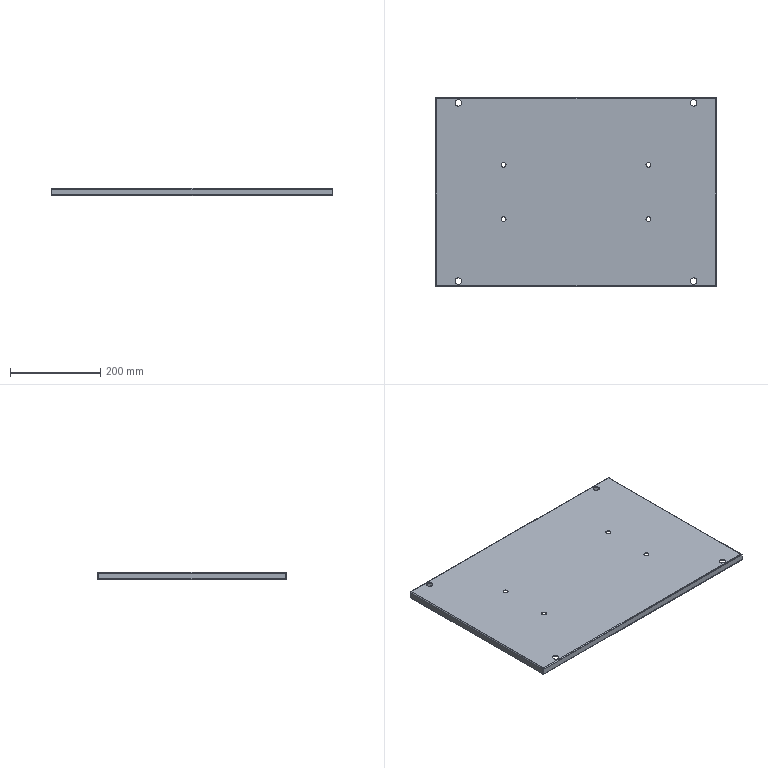Part | STEP file | SX-023-01 | 1 solid | 104 faces | box 620.667 x 418.001 x 17 mm | volume 629172 mm3 | plane 54 | cylinder 38 | spline 12 | commonest cylinder face diameters 0.4 x8 4.4 x8 11 x8 14 x8 18 x6